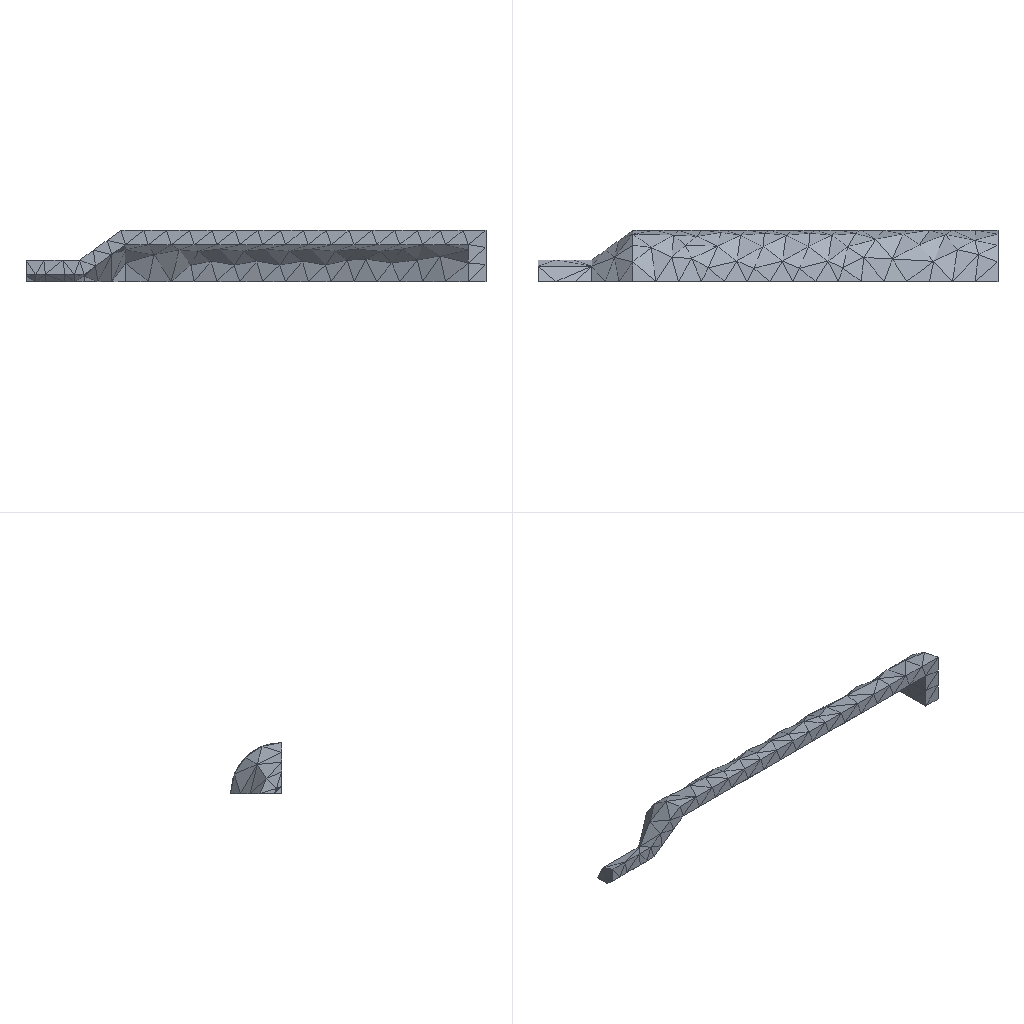Simulation study | ansys workbench
Ansys APDL input file, long lists of numbers shortened:
/batch
/config,noeldb,1     ! force off writing results to database
*get,_wallstrt,active,,time,wall
! ANSYS input file written by Workbench version 2022 R1
! File used for geometry attach:
/title,wbnew--____ (C5)
! ****** Begin Custom Load Command Snippet ******
/COM, ACT Extensions:
/COM,     LSDYNA, 2021.1
/COM,
! ****** End   Custom Load Command Snippet ******
*DIM,_wb_ProjectScratch_dir,string,248
_wb_ProjectScratch_dir(1) = ''
*DIM,_wb_SolverFiles_dir,string,248
_wb_SolverFiles_dir(1) = ''
*DIM,_wb_userfiles_dir,string,248
_wb_userfiles_dir(1) = ''
/com,--- Data in consistent NMM units. See Solving Units in the help system for more information.
/units,MPA
/nopr
/wb,file,start              !  signify a WB generated input file
/prep7
! Turn off shape checking because checks already performed inside WB mesher.
! See help system for more information.
SHPP,OFF,,NOWARN
/nolist
etcon,set             ! allow ANSYS to choose best KEYOP's for 180x elements, resets any applicable keyopt to MAPDL defaults
/com,*********** Nodes for the whole assembly ***********
nblock,3,,986
(1i9,3e20.9e3)
        1     1.301000000E+03     0.000000000E+00     0.000000000E+00
! (896 more lines like these left out)
-1
/wb,elem,start            !  set before creation of elements
/com,*********** Elements for Body 1 "__3-FreeParts|__-__5" ***********
et,1,187
eblock,19,solid,,373
(19i9)
        1        1        1        1        0        0        0        0       10        0        1      127      174      136      137      764      810      759      760
! (745 more lines like these left out)
-1
/wb,elem,end               !  done creating elements
/com,*********** Send User Defined Coordinate System(s) ***********
csys,0
toffst,273.15,  ! Temperature offset from absolute zero
/com,*********** Set Reference Temperature ***********
tref,22.
/wb,mat,start              !  starting to send materials
/com,*********** Send Materials ***********
Temperature = 'TEMP' ! Temperature
MP,DENS,1,7.85e-09,	! tonne mm^-3
MP,ALPX,1,1.2e-05,	! C^-1
MP,C,1,434000000,	! mm^2 s^-2 C^-1
MP,KXX,1,60.5,	! tonne mm s^-3 C^-1
MP,RSVX,1,0.00017,	! ohm mm
MP,EX,1,200000,	! tonne s^-2 mm^-1
MP,NUXY,1,0.3,
MP,MURX,1,10000,
/wb,mat,end                !  done sending materials
!************************* Model Summary ********************
!__3-FreeParts|__-__5,	结构钢,	matid,	1
!************************* End Model Summary ********************
! get the diagonal of the bounding box. Needed later for other things
*get,_xmin,node,,mnloc,x
*get,_ymin,node,,mnloc,y
*get,_zmin,node,,mnloc,z
*get,_xmax,node,,mxloc,x
*get,_ymax,node,,mxloc,y
*get,_zmax,node,,mxloc,z
_ASMDIAG=(_xmax-_xmin)*(_xmax-_xmin)+(_ymax-_ymin)*(_ymax-_ymin)+(_zmax-_zmin)*(_zmax-_zmin)
_ASMDIAG=SQRT(_ASMDIAG)
/wb,contact,start          !  starting to send contact
/wb,contact,end            !  done creating contacts
/golist
/wb,load,start             !  starting to send loads
/com,*********** Fixed Supports ***********
CMBLOCK,_FIXEDSU,NODE,       27
(8i10)
         1         2         3         4         5         6         7         8
         9        10       177       178       180       181       184       185
       186       192       193       197       198       201       202       203
       207       211       216
cmsel,s,_FIXEDSU
d,all,all
nsel,all
/com,*********** Define Pressure Using Surface Effect Elements "__" ***********
et,2,154
eblock,10,,,106
(15i9)
      720        2        2        2        0        8        9      142      142      211      219      142      215
! (105 more lines like these left out)
-1
esel,s,type,,2
keyop,2,7,0                ! Use deformed area for application of load
esel,all
/com,*********** Define Pressure Using Surface Effect Elements "__ 2" ***********
et,3,154
eblock,10,,,82
(15i9)
      826        3        3        3        0       70       72       95       95      519      528       95      521
! (81 more lines like these left out)
-1
esel,s,type,,3
keyop,3,7,0                ! Use deformed area for application of load
esel,all
esel,all
/gst,on,on
fini
*get,_numnode,node,0,count
*get,_numelem,elem,0,count
*get, _MAXELEMNUM, elem, 0, NUM, MAX
*get, _MAXNODENUM, node, 0, NUM, MAX
*get, _MAXELEMTYPE, etyp, 0, NUM, MAX
*get, _MAXREALCONST, real, 0, NUM, MAX
/go
/wb,load,end               !  done creating loads
/com,--- Number of total nodes = %_numnode%
/com,--- Number of contact elements = 188
/com,--- Number of spring elements = 0
/com,--- Number of bearing elements = 0
/com,--- Number of solid elements = 373
/com,--- Number of condensed parts = 0
/com,--- Number of total elements = %_numelem%
*get,_wallbsol,active,,time,wall
/com,****************************************************************************
/com,*************************    SOLUTION       ********************************
/com,****************************************************************************
/solu
antype,0                   ! static analysis
_thickRatio=  0     ! Ratio of thick parts in the model
eqsl,sparse,,,,,1
cntr,print,1               ! print out contact info and also make no initial contact an error
dmpoption,emat,no             ! Don't combine emat file for DANSYS
dmpoption,esav,no             ! Don't combine esav file for DANSYS
nldiag,cont,iter           ! print out contact info each equilibrium iteration
rescontrol,,none                 ! Do not keep any restart files
/com,****************************************************
/com,******************* SOLVE FOR LS 1 OF 1 ****************
esel,s,type,,2
nsle
sf,all,pres,20.
esel,s,type,,3
nsle
sf,all,pres,60.
nsel,all
esel,all
esel,all
/nopr
/gopr
nsub,1,1,1
time,1.
outres,erase
outres,all,none
outres,nsol,all,
outres,rsol,all
outres,eangl,all
outres,etmp,all
outres,veng,all
outres,strs,all,
outres,epel,all,
outres,eppl,all,
outres,cont,all,
! *********** WB SOLVE COMMAND ***********
! check interactive state
*get,ANSINTER_,active,,int
*if,ANSINTER_,ne,0,then
/eof
*endif
solve
/com *************** Write FE CONNECTORS *********
CEWRITE,file,ce,,INTE
/com,****************************************************
/com,*************** FINISHED SOLVE FOR LS 1 *************
*get,_wallasol,active,,time,wall
/nopr
*get,_numnode,node,0,count
*get,_numelem,elem,0,count
*get, _MAXELEMNUM, elem, 0, NUM, MAX
*get, _MAXNODENUM, node, 0, NUM, MAX,,,INTERNAL
*get, _MAXELEMTYPE, etyp, 0, NUM, MAX
*get, _MAXREALCONST, real, 0, NUM, MAX
/gopr
/post1
xmlo,ENCODING,ISO-8859-1
xmlo,parm
/xml,parm,xml
fini
/gopr
*get,_walldone,active,,time,wall
_preptime=(_wallbsol-_wallstrt)*3600
_solvtime=(_wallasol-_wallbsol)*3600
_posttime=(_walldone-_wallasol)*3600
_totaltim=(_walldone-_wallstrt)*3600
*get,_dlbratio,active,0,solu,dlbr
*get,_combtime,active,0,solu,comb
*get,_ssmode,active,0,solu,ssmm
*get,_ndofs,active,0,solu,ndof
*get,_sol_end_time,active,0,set,time
*if,_sol_end_time,eq,1.,then
/fclean				!clean distributed files
*endif
/com,--- Total number of nodes = %_numnode%
/com,--- Total number of elements = %_numelem%
/com,--- Element load balance ratio = %_dlbratio%
/com,--- Time to combine distributed files = %_combtime%
/com,--- Sparse memory mode = %_ssmode%
/com,--- Number of DOF = %_ndofs%
/wb,file,end               ! done with WB generated input